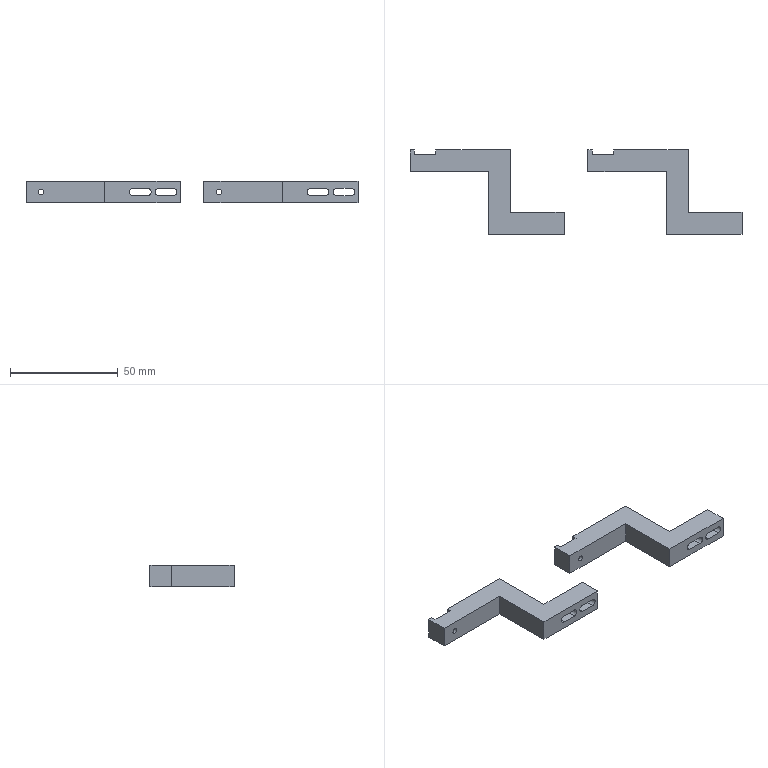CAM job | NX | 3+2 milling, drilling | part box 154 x 39 x 10 mm | stock box 158 x 45 x 12 mm
Tools:
number,name,description,diameter,corner_radius,flute_length,length,flutes
17,D2,平底铣刀-粗,2.0,0.0,50.0,75.0,2
6,D6,平底铣刀-粗,6.0,0.0,25.0,75.0,2
9,D10,平底铣刀-粗,10.0,0.0,35.0,75.0,2
7,D6-J,平底铣刀-精,6.0,0.0,25.0,75.0,2
10,D10-J,平底铣刀-精,10.0,0.0,35.0,75.0,2
1,D80R0.8飞刀,圆鼻刀-粗,80.0,0.8,50.0,75.0,2
1,D80R0.8飞刀-J,圆鼻刀-精,80.0,0.8,50.0,75.0,2
2,D6倒角刀,倒角刀,6.0,0.0,3.0,25.0,2
20,M3X0.5,丝锥,2.5,0.0,35.0,50.0,2
12,钻头2.5,Twist Drill 2.5 mm,2.5,0.0,30.0,32.0,2
Operations:
program,operation,operation_type,tool,method,geometry_group,spindle_rpm,surface_speed,feed_per_tooth,feed_cut,feed_plunge,cut_length_mm,path_length_mm,cut_time_min,machine_time_min
B,底壁铣飞面一刀开粗_COPY,VolumeBased25DMillingOperation,D80R0.8飞刀,分层开粗-切深K-步距G,W-B,5000.0,1256.637,0.3,3000.0,100.0,2884.134,5723.512,0.9614,1.245
B,底壁铣飞面一刀精光_COPY,VolumeBased25DMillingOperation,D80R0.8飞刀-J,侧刃精光-切深K-步距G,W-B,5000.0,1256.637,0.1,1000.0,100.0,261.998,297.998,0.262,0.2656
B,底壁粗_3,VolumeBased25DMillingOperation,D10,METHOD,W-B,6000.0,113.0,0.2083,3500.0,100.0,18455.6,19647.987,5.273,5.392
B,腰槽粗_1,VolumeBased25DMillingOperation,D2,METHOD,W-B,6000.0,37.699,0.125,1500.0,100.0,7608.649,7921.781,5.072,5.104
B,腰槽精_1,VolumeBased25DMillingOperation,D2,METHOD,W-B,6000.0,37.699,0.05,600.0,100.0,555.143,1030.343,0.9252,0.9728
B,钻倒角_2,Operation,D6倒角刀,METHOD,W-B,8000.0,150.796,0.0312,500.0,0.0,9.5,202.554,0.019,0.0383
B,平面去毛刺6X45L_COPY,SurfaceContour,D6倒角刀,爬面_倒角-切深0-步距G,W-B,6500.0,122.519,0.1154,1500.0,100.0,558.692,939.047,0.3725,0.4105
B,底精_3,VolumeBased25DMillingOperation,D6-J,METHOD,W-B,6000.0,113.0,0.2083,1200.0,100.0,334.2,613.1,0.2785,0.3064
B,底侧精_5,VolumeBased25DMillingOperation,D6-J,METHOD,W-B,6000.0,113.0,0.2083,1200.0,100.0,157.933,948.598,0.1316,0.2107
A,顶面,FaceMilling,D80R0.8飞刀,侧刃精光-切深K-步距G,W-A,5000.0,1256.637,0.1,1000.0,100.0,248.0,284.0,0.248,0.2516
A,外形粗_2,VolumeBased25DMillingOperation,D10,METHOD,W-A,8000.0,251.327,0.3125,5000.0,80.0,19897.675,20136.275,3.979,4.003
A,底壁粗_1,VolumeBased25DMillingOperation,D10,METHOD,W-A,6000.0,113.0,0.2083,3500.0,100.0,13119.6,14310.135,3.748,3.868
A,底壁粗_2,VolumeBased25DMillingOperation,D6,METHOD,W-A,6000.0,113.0,0.2083,3500.0,100.0,370.0,589.043,0.1057,0.1276
A,打点-深0.8,Operation,D6倒角刀,NONE,W-A,8000.0,150.796,0.0312,500.0,90.0,3.6,134.706,0.0072,0.0203
A,通孔-M3螺纹底孔,Operation,钻头2.5,NONE,W-A,3000.0,23.562,0.05,300.0,90.0,29.502,186.51,0.0983,0.114
A,底精_1,VolumeBased25DMillingOperation,D6-J,METHOD,W-A,6000.0,113.0,0.2083,1200.0,100.0,242.2,518.2,0.2018,0.2294
A,底精_2,VolumeBased25DMillingOperation,D6-J,METHOD,W-A,6000.0,113.0,0.2083,1200.0,100.0,84.2,252.2,0.0702,0.087
A,仅选体,SurfaceContour,D6倒角刀,METHOD,W-A,8000.0,150.796,0.1875,3000.0,100.0,606.448,1355.987,0.2021,0.2771
A,钻倒角_1,Operation,D6倒角刀,METHOD,W-A,8000.0,150.796,0.0312,500.0,0.0,9.5,148.554,0.019,0.0329
A,通孔-攻牙M3,Operation,M3X0.5,METHOD,W-A,800.0,6.283,0.0003,0.5,90.0,24.0,175.506,48.0,48.015
A,底侧精_3,VolumeBased25DMillingOperation,D6-J,METHOD,W-A,6000.0,113.0,0.2083,1200.0,100.0,157.933,948.598,0.1316,0.2107
A,底侧精_4,VolumeBased25DMillingOperation,D6-J,METHOD,W-A,6000.0,113.0,0.2083,1200.0,100.0,80.666,247.296,0.0672,0.0839
A,外形半精_2,VolumeBased25DMillingOperation,D10-J,METHOD,W-A,8000.0,251.327,0.0625,1000.0,100.0,797.747,1463.422,0.7977,0.8643